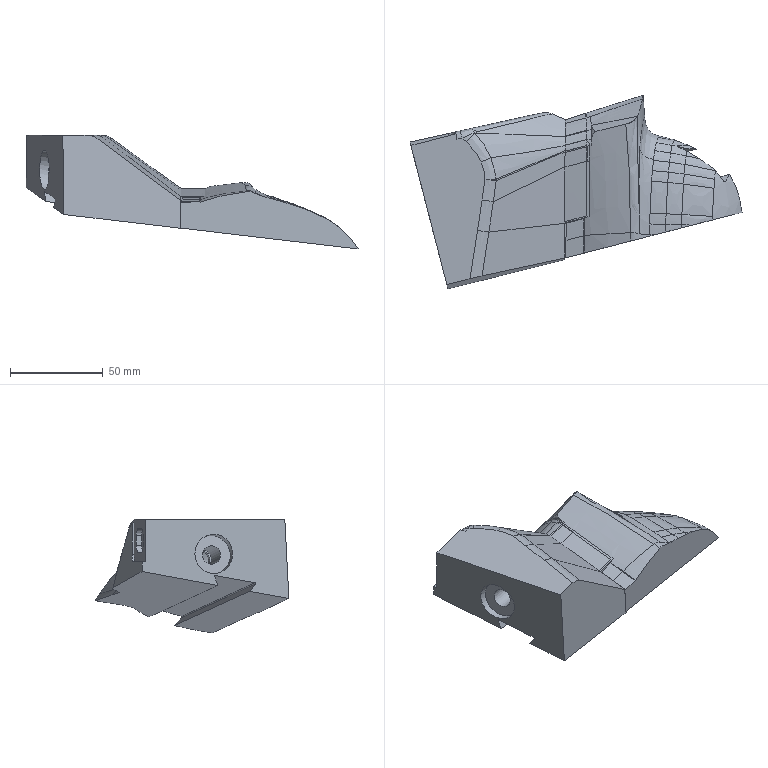Part | STEP file | 车灯-后视镜_id334_x_t | 1 solid | 137 faces | box 178.639 x 104.251 x 61.239 mm | volume 236319 mm3 | spline 79 | plane 31 | other 14 | cylinder 11 | cone 2 | commonest cylinder face diameters 8 x6 4.3 x1 5 x1 8.5 x1 10 x1 21 x1